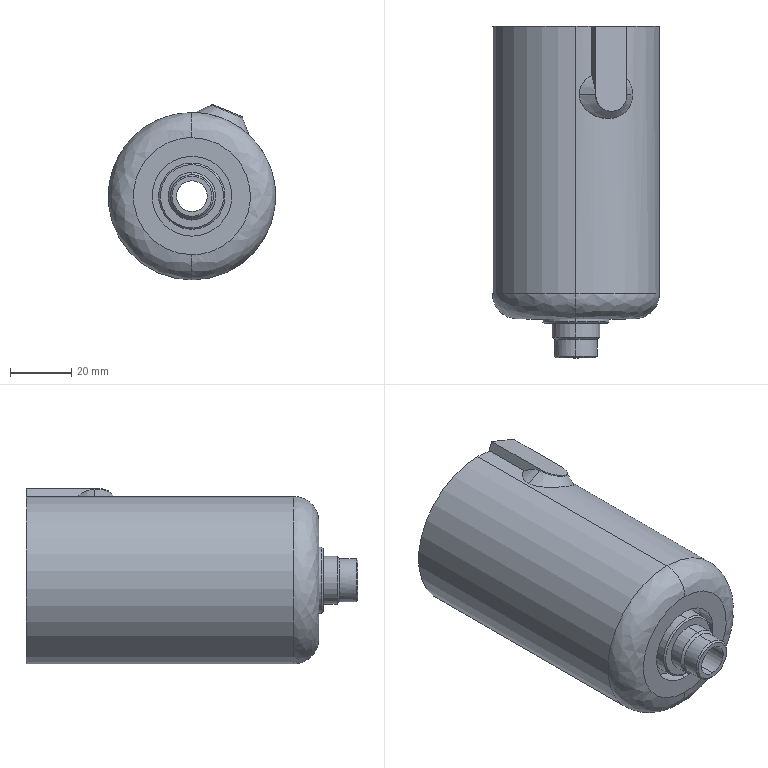Part | STEP file | HI_BF4000-A By | 1 solid | 42 faces | box 54.5 x 108 x 57.228 mm | volume 40033 mm3 | cylinder 17 | plane 12 | cone 9 | spline 4 | commonest cylinder face diameters 10 x2 14 x2 15.5 x2 21.6 x2 26 x2 30 x2